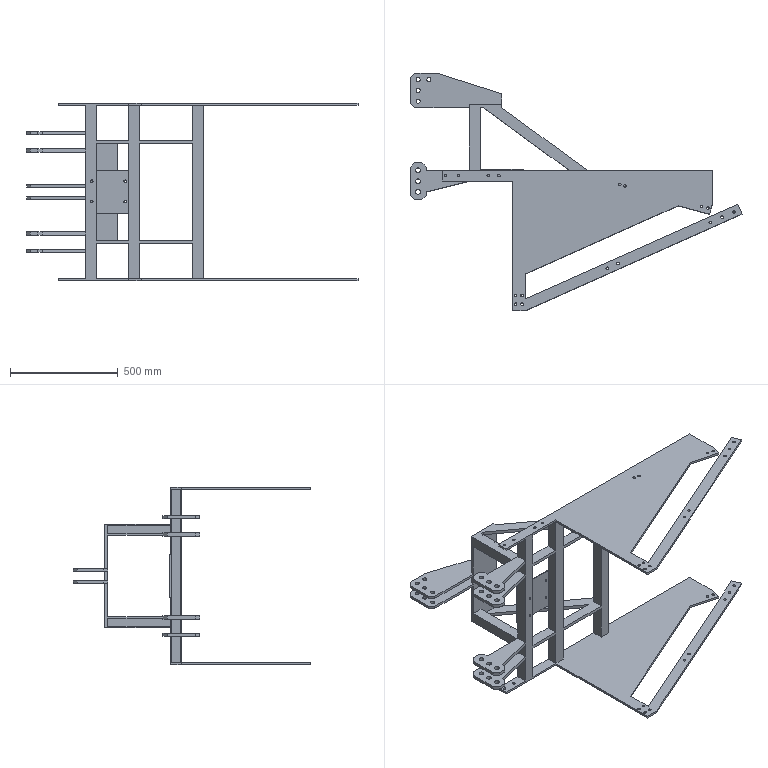Part | SolidWorks | features ICE 29, Extrusion 1 | 2 solids | 295 faces | box 1540 x 1103 x 825 mm | volume 15486897 mm3 | plane 183 | cylinder 112 | commonest cylinder face diameters 12 x72 22 x24 19.3 x16